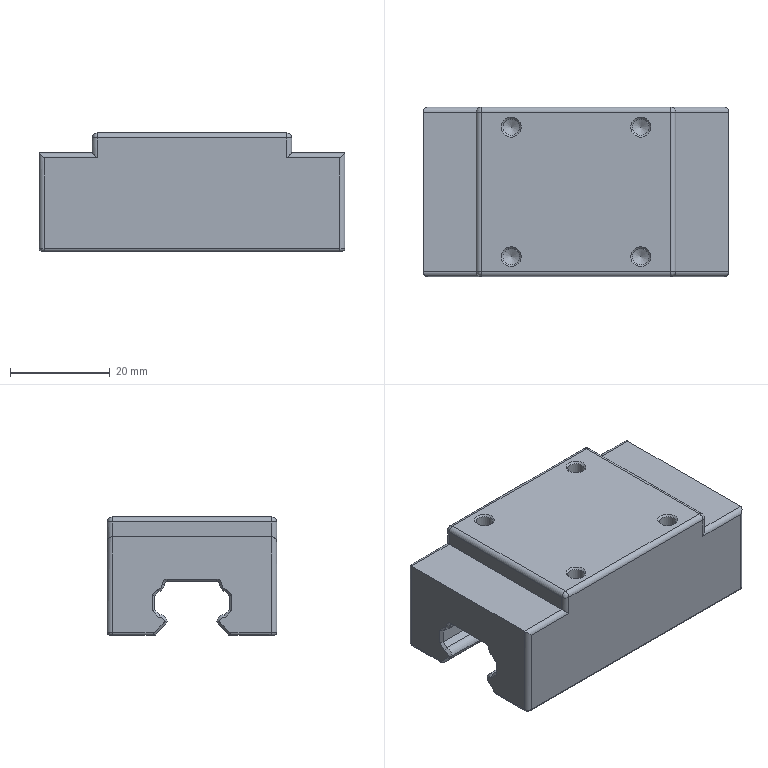Part | STEP file | Tube feed_id594_x_t | 1 solid | 104 faces | box 61.4 x 34 x 23.7 mm | volume 37642 mm3 | plane 38 | cylinder 34 | cone 24 | sphere 4 | spline 4 | commonest cylinder face diameters 2 x16 1 x8 3 x6 3.3 x4